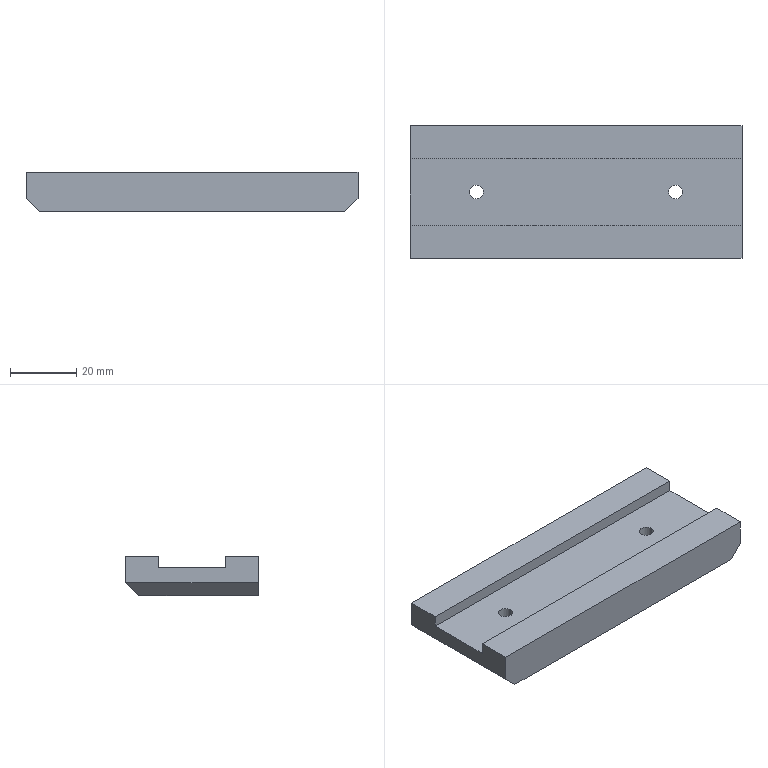Part | STEP file | X77-02103 | 1 solid | 17 faces | box 100 x 40 x 12 mm | volume 39367 mm3 | plane 13 | cylinder 4 | commonest cylinder face diameters 4.2 x4
STEP:
#1=CARTESIAN_POINT('',(-32.1,70.,0.));
#2=VERTEX_POINT('',#1);
#3=CARTESIAN_POINT('',(-27.9,70.,0.));
#4=VERTEX_POINT('',#3);
#5=CARTESIAN_POINT('',(-30.,70.,0.));
#6=DIRECTION('',(0.,0.,1.));
#7=DIRECTION('',(1.,0.,0.));
#8=AXIS2_PLACEMENT_3D('',#5,#6,#7);
#9=CIRCLE('',#8,2.1);
#10=EDGE_CURVE('',#2,#4,#9,.T.);
#11=ORIENTED_EDGE('',*,*,#10,.F.);
#12=CARTESIAN_POINT('',(-32.1,70.,8.5));
#13=VERTEX_POINT('',#12);
#14=CARTESIAN_POINT('',(-32.1,70.,8.5));
#15=DIRECTION('',(0.,0.,1.));
#16=VECTOR('',#15,1000.);
#17=LINE('',#14,#16);
#18=EDGE_CURVE('',#2,#13,#17,.T.);
#19=ORIENTED_EDGE('',*,*,#18,.T.);
#20=CARTESIAN_POINT('',(-27.9,70.,8.5));
#21=VERTEX_POINT('',#20);
#22=CARTESIAN_POINT('',(-30.,70.,8.5));
#23=DIRECTION('',(0.,0.,1.));
#24=DIRECTION('',(1.,0.,0.));
#25=AXIS2_PLACEMENT_3D('',#22,#23,#24);
#26=CIRCLE('',#25,2.1);
#27=EDGE_CURVE('',#13,#21,#26,.T.);
#28=ORIENTED_EDGE('',*,*,#27,.T.);
#29=CARTESIAN_POINT('',(-27.9,70.,8.5));
#30=DIRECTION('',(0.,0.,1.));
#31=VECTOR('',#30,1000.);
#32=LINE('',#29,#31);
#33=EDGE_CURVE('',#4,#21,#32,.T.);
#34=ORIENTED_EDGE('',*,*,#33,.F.);
#35=EDGE_LOOP('',(#11,#19,#28,#34));
#36=FACE_OUTER_BOUND('',#35,.T.);
#37=CARTESIAN_POINT('',(-30.,70.,8.5));
#38=DIRECTION('',(0.,0.,1.));
#39=DIRECTION('',(1.,0.,0.));
#40=AXIS2_PLACEMENT_3D('',#37,#38,#39);
#41=CYLINDRICAL_SURFACE('',#40,2.1);
#42=ADVANCED_FACE('',(#36),#41,.F.);
#43=CARTESIAN_POINT('',(27.9,70.,0.));
#44=VERTEX_POINT('',#43);
#45=CARTESIAN_POINT('',(32.1,70.,0.));
#46=VERTEX_POINT('',#45);
#47=CARTESIAN_POINT('',(30.,70.,0.));
#48=DIRECTION('',(0.,0.,1.));
#49=DIRECTION('',(1.,0.,0.));
#50=AXIS2_PLACEMENT_3D('',#47,#48,#49);
#51=CIRCLE('',#50,2.1);
#52=EDGE_CURVE('',#44,#46,#51,.T.);
#53=ORIENTED_EDGE('',*,*,#52,.F.);
#54=CARTESIAN_POINT('',(27.9,70.,8.5));
#55=VERTEX_POINT('',#54);
#56=CARTESIAN_POINT('',(27.9,70.,8.5));
#57=DIRECTION('',(0.,0.,1.));
#58=VECTOR('',#57,1000.);
#59=LINE('',#56,#58);
#60=EDGE_CURVE('',#44,#55,#59,.T.);
#61=ORIENTED_EDGE('',*,*,#60,.T.);
#62=CARTESIAN_POINT('',(32.1,70.,8.5));
#63=VERTEX_POINT('',#62);
#64=CARTESIAN_POINT('',(30.,70.,8.5));
#65=DIRECTION('',(0.,0.,1.));
#66=DIRECTION('',(1.,0.,0.));
#67=AXIS2_PLACEMENT_3D('',#64,#65,#66);
#68=CIRCLE('',#67,2.1);
#69=EDGE_CURVE('',#55,#63,#68,.T.);
#70=ORIENTED_EDGE('',*,*,#69,.T.);
#71=CARTESIAN_POINT('',(32.1,70.,8.5));
#72=DIRECTION('',(0.,0.,1.));
#73=VECTOR('',#72,1000.);
#74=LINE('',#71,#73);
#75=EDGE_CURVE('',#46,#63,#74,.T.);
#76=ORIENTED_EDGE('',*,*,#75,.F.);
#77=EDGE_LOOP('',(#53,#61,#70,#76));
#78=FACE_OUTER_BOUND('',#77,.T.);
#79=CARTESIAN_POINT('',(30.,70.,8.5));
#80=DIRECTION('',(0.,0.,1.));
#81=DIRECTION('',(1.,0.,0.));
#82=AXIS2_PLACEMENT_3D('',#79,#80,#81);
#83=CYLINDRICAL_SURFACE('',#82,2.1);
#84=ADVANCED_FACE('',(#78),#83,.F.);
#85=CARTESIAN_POINT('',(-50.,60.,12.));
#86=VERTEX_POINT('',#85);
#87=CARTESIAN_POINT('',(50.,60.,12.));
#88=VERTEX_POINT('',#87);
#89=CARTESIAN_POINT('',(-50.,60.,12.));
#90=DIRECTION('',(1.,0.,0.));
#91=VECTOR('',#90,1000.);
#92=LINE('',#89,#91);
#93=EDGE_CURVE('',#86,#88,#92,.T.);
#94=ORIENTED_EDGE('',*,*,#93,.F.);
#95=CARTESIAN_POINT('',(-50.,50.,12.));
#96=VERTEX_POINT('',#95);
#97=CARTESIAN_POINT('',(-50.,90.,12.));
#98=DIRECTION('',(0.,-1.,0.));
#99=VECTOR('',#98,1000.);
#100=LINE('',#97,#99);
#101=EDGE_CURVE('',#86,#96,#100,.T.);
#102=ORIENTED_EDGE('',*,*,#101,.T.);
#103=CARTESIAN_POINT('',(50.,50.,12.));
#104=VERTEX_POINT('',#103);
#105=CARTESIAN_POINT('',(-50.,50.,12.));
#106=DIRECTION('',(1.,0.,0.));
#107=VECTOR('',#106,1000.);
#108=LINE('',#105,#107);
#109=EDGE_CURVE('',#96,#104,#108,.T.);
#110=ORIENTED_EDGE('',*,*,#109,.T.);
#111=CARTESIAN_POINT('',(50.,90.,12.));
#112=DIRECTION('',(0.,1.,0.));
#113=VECTOR('',#112,1000.);
#114=LINE('',#111,#113);
#115=EDGE_CURVE('',#104,#88,#114,.T.);
#116=ORIENTED_EDGE('',*,*,#115,.T.);
#117=EDGE_LOOP('',(#94,#102,#110,#116));
#118=FACE_OUTER_BOUND('',#117,.T.);
#119=CARTESIAN_POINT('',(-50.,50.,12.));
#120=DIRECTION('',(0.,0.,1.));
#121=DIRECTION('',(1.,0.,0.));
#122=AXIS2_PLACEMENT_3D('',#119,#120,#121);
#123=PLANE('',#122);
#124=ADVANCED_FACE('',(#118),#123,.T.);
#125=ORIENTED_EDGE('',*,*,#101,.F.);
#126=CARTESIAN_POINT('',(-50.,60.,8.5));
#127=VERTEX_POINT('',#126);
#128=CARTESIAN_POINT('',(-50.,60.,8.5));
#129=DIRECTION('',(0.,0.,1.));
#130=VECTOR('',#129,1000.);
#131=LINE('',#128,#130);
#132=EDGE_CURVE('',#127,#86,#131,.T.);
#133=ORIENTED_EDGE('',*,*,#132,.F.);
#134=CARTESIAN_POINT('',(-50.,80.,8.5));
#135=VERTEX_POINT('',#134);
#136=CARTESIAN_POINT('',(-50.,80.,8.5));
#137=DIRECTION('',(0.,-1.,0.));
#138=VECTOR('',#137,1000.);
#139=LINE('',#136,#138);
#140=EDGE_CURVE('',#135,#127,#139,.T.);
#141=ORIENTED_EDGE('',*,*,#140,.F.);
#142=CARTESIAN_POINT('',(-50.,80.,12.));
#143=VERTEX_POINT('',#142);
#144=CARTESIAN_POINT('',(-50.,80.,8.5));
#145=DIRECTION('',(0.,0.,1.));
#146=VECTOR('',#145,1000.);
#147=LINE('',#144,#146);
#148=EDGE_CURVE('',#135,#143,#147,.T.);
#149=ORIENTED_EDGE('',*,*,#148,.T.);
#150=CARTESIAN_POINT('',(-50.,90.,12.));
#151=VERTEX_POINT('',#150);
#152=CARTESIAN_POINT('',(-50.,90.,12.));
#153=DIRECTION('',(0.,-1.,0.));
#154=VECTOR('',#153,1000.);
#155=LINE('',#152,#154);
#156=EDGE_CURVE('',#151,#143,#155,.T.);
#157=ORIENTED_EDGE('',*,*,#156,.F.);
#158=CARTESIAN_POINT('',(-50.,90.,4.));
#159=VERTEX_POINT('',#158);
#160=CARTESIAN_POINT('',(-50.,90.,12.));
#161=DIRECTION('',(0.,0.,-1.));
#162=VECTOR('',#161,1000.);
#163=LINE('',#160,#162);
#164=EDGE_CURVE('',#151,#159,#163,.T.);
#165=ORIENTED_EDGE('',*,*,#164,.T.);
#166=CARTESIAN_POINT('',(-50.,50.,4.));
#167=VERTEX_POINT('',#166);
#168=CARTESIAN_POINT('',(-50.,90.,4.));
#169=DIRECTION('',(0.,-1.,0.));
#170=VECTOR('',#169,1000.);
#171=LINE('',#168,#170);
#172=EDGE_CURVE('',#159,#167,#171,.T.);
#173=ORIENTED_EDGE('',*,*,#172,.T.);
#174=CARTESIAN_POINT('',(-50.,50.,12.));
#175=DIRECTION('',(0.,0.,-1.));
#176=VECTOR('',#175,1000.);
#177=LINE('',#174,#176);
#178=EDGE_CURVE('',#96,#167,#177,.T.);
#179=ORIENTED_EDGE('',*,*,#178,.F.);
#180=EDGE_LOOP('',(#125,#133,#141,#149,#157,#165,#173,#179));
#181=FACE_OUTER_BOUND('',#180,.T.);
#182=CARTESIAN_POINT('',(-50.,90.,12.));
#183=DIRECTION('',(1.,0.,0.));
#184=DIRECTION('',(0.,1.,0.));
#185=AXIS2_PLACEMENT_3D('',#182,#183,#184);
#186=PLANE('',#185);
#187=ADVANCED_FACE('',(#181),#186,.F.);
#188=ORIENTED_EDGE('',*,*,#178,.T.);
#189=CARTESIAN_POINT('',(-46.,50.,0.));
#190=VERTEX_POINT('',#189);
#191=CARTESIAN_POINT('',(-50.,50.,4.));
#192=DIRECTION('',(0.7071,0.,-0.7071));
#193=VECTOR('',#192,1000.);
#194=LINE('',#191,#193);
#195=EDGE_CURVE('',#167,#190,#194,.T.);
#196=ORIENTED_EDGE('',*,*,#195,.T.);
#197=CARTESIAN_POINT('',(46.,50.,0.));
#198=VERTEX_POINT('',#197);
#199=CARTESIAN_POINT('',(-50.,50.,0.));
#200=DIRECTION('',(1.,0.,0.));
#201=VECTOR('',#200,1000.);
#202=LINE('',#199,#201);
#203=EDGE_CURVE('',#190,#198,#202,.T.);
#204=ORIENTED_EDGE('',*,*,#203,.T.);
#205=CARTESIAN_POINT('',(50.,50.,4.));
#206=VERTEX_POINT('',#205);
#207=CARTESIAN_POINT('',(50.,50.,4.));
#208=DIRECTION('',(0.7071,0.,0.7071));
#209=VECTOR('',#208,1000.);
#210=LINE('',#207,#209);
#211=EDGE_CURVE('',#198,#206,#210,.T.);
#212=ORIENTED_EDGE('',*,*,#211,.T.);
#213=CARTESIAN_POINT('',(50.,50.,12.));
#214=DIRECTION('',(0.,0.,-1.));
#215=VECTOR('',#214,1000.);
#216=LINE('',#213,#215);
#217=EDGE_CURVE('',#104,#206,#216,.T.);
#218=ORIENTED_EDGE('',*,*,#217,.F.);
#219=ORIENTED_EDGE('',*,*,#109,.F.);
#220=EDGE_LOOP('',(#188,#196,#204,#212,#218,#219));
#221=FACE_OUTER_BOUND('',#220,.T.);
#222=CARTESIAN_POINT('',(-50.,50.,12.));
#223=DIRECTION('',(0.,1.,0.));
#224=DIRECTION('',(0.,0.,1.));
#225=AXIS2_PLACEMENT_3D('',#222,#223,#224);
#226=PLANE('',#225);
#227=ADVANCED_FACE('',(#221),#226,.F.);
#228=CARTESIAN_POINT('',(50.,60.,8.5));
#229=VERTEX_POINT('',#228);
#230=CARTESIAN_POINT('',(50.,80.,8.5));
#231=VERTEX_POINT('',#230);
#232=CARTESIAN_POINT('',(50.,80.,8.5));
#233=DIRECTION('',(0.,1.,0.));
#234=VECTOR('',#233,1000.);
#235=LINE('',#232,#234);
#236=EDGE_CURVE('',#229,#231,#235,.T.);
#237=ORIENTED_EDGE('',*,*,#236,.F.);
#238=CARTESIAN_POINT('',(50.,60.,8.5));
#239=DIRECTION('',(0.,0.,1.));
#240=VECTOR('',#239,1000.);
#241=LINE('',#238,#240);
#242=EDGE_CURVE('',#229,#88,#241,.T.);
#243=ORIENTED_EDGE('',*,*,#242,.T.);
#244=ORIENTED_EDGE('',*,*,#115,.F.);
#245=ORIENTED_EDGE('',*,*,#217,.T.);
#246=CARTESIAN_POINT('',(50.,90.,4.));
#247=VERTEX_POINT('',#246);
#248=CARTESIAN_POINT('',(50.,90.,4.));
#249=DIRECTION('',(0.,1.,0.));
#250=VECTOR('',#249,1000.);
#251=LINE('',#248,#250);
#252=EDGE_CURVE('',#206,#247,#251,.T.);
#253=ORIENTED_EDGE('',*,*,#252,.T.);
#254=CARTESIAN_POINT('',(50.,90.,12.));
#255=VERTEX_POINT('',#254);
#256=CARTESIAN_POINT('',(50.,90.,12.));
#257=DIRECTION('',(0.,0.,-1.));
#258=VECTOR('',#257,1000.);
#259=LINE('',#256,#258);
#260=EDGE_CURVE('',#255,#247,#259,.T.);
#261=ORIENTED_EDGE('',*,*,#260,.F.);
#262=CARTESIAN_POINT('',(50.,80.,12.));
#263=VERTEX_POINT('',#262);
#264=CARTESIAN_POINT('',(50.,90.,12.));
#265=DIRECTION('',(0.,1.,0.));
#266=VECTOR('',#265,1000.);
#267=LINE('',#264,#266);
#268=EDGE_CURVE('',#263,#255,#267,.T.);
#269=ORIENTED_EDGE('',*,*,#268,.F.);
#270=CARTESIAN_POINT('',(50.,80.,8.5));
#271=DIRECTION('',(0.,0.,1.));
#272=VECTOR('',#271,1000.);
#273=LINE('',#270,#272);
#274=EDGE_CURVE('',#231,#263,#273,.T.);
#275=ORIENTED_EDGE('',*,*,#274,.F.);
#276=EDGE_LOOP('',(#237,#243,#244,#245,#253,#261,#269,#275));
#277=FACE_OUTER_BOUND('',#276,.T.);
#278=CARTESIAN_POINT('',(50.,90.,12.));
#279=DIRECTION('',(-1.,0.,0.));
#280=DIRECTION('',(0.,0.,1.));
#281=AXIS2_PLACEMENT_3D('',#278,#279,#280);
#282=PLANE('',#281);
#283=ADVANCED_FACE('',(#277),#282,.F.);
#284=ORIENTED_EDGE('',*,*,#260,.T.);
#285=CARTESIAN_POINT('',(-50.,90.,4.));
#286=DIRECTION('',(-1.,0.,0.));
#287=VECTOR('',#286,1000.);
#288=LINE('',#285,#287);
#289=EDGE_CURVE('',#247,#159,#288,.T.);
#290=ORIENTED_EDGE('',*,*,#289,.T.);
#291=ORIENTED_EDGE('',*,*,#164,.F.);
#292=CARTESIAN_POINT('',(-50.,90.,12.));
#293=DIRECTION('',(-1.,0.,0.));
#294=VECTOR('',#293,1000.);
#295=LINE('',#292,#294);
#296=EDGE_CURVE('',#255,#151,#295,.T.);
#297=ORIENTED_EDGE('',*,*,#296,.F.);
#298=EDGE_LOOP('',(#284,#290,#291,#297));
#299=FACE_OUTER_BOUND('',#298,.T.);
#300=CARTESIAN_POINT('',(-50.,90.,12.));
#301=DIRECTION('',(0.,-1.,0.));
#302=DIRECTION('',(0.,0.,-1.));
#303=AXIS2_PLACEMENT_3D('',#300,#301,#302);
#304=PLANE('',#303);
#305=ADVANCED_FACE('',(#299),#304,.F.);
#306=CARTESIAN_POINT('',(-50.,80.,12.));
#307=DIRECTION('',(-1.,0.,0.));
#308=VECTOR('',#307,1000.);
#309=LINE('',#306,#308);
#310=EDGE_CURVE('',#263,#143,#309,.T.);
#311=ORIENTED_EDGE('',*,*,#310,.F.);
#312=ORIENTED_EDGE('',*,*,#268,.T.);
#313=ORIENTED_EDGE('',*,*,#296,.T.);
#314=ORIENTED_EDGE('',*,*,#156,.T.);
#315=EDGE_LOOP('',(#311,#312,#313,#314));
#316=FACE_OUTER_BOUND('',#315,.T.);
#317=CARTESIAN_POINT('',(-50.,50.,12.));
#318=DIRECTION('',(0.,0.,1.));
#319=DIRECTION('',(1.,0.,0.));
#320=AXIS2_PLACEMENT_3D('',#317,#318,#319);
#321=PLANE('',#320);
#322=ADVANCED_FACE('',(#316),#321,.T.);
#323=CARTESIAN_POINT('',(-30.,70.,0.));
#324=DIRECTION('',(0.,0.,1.));
#325=DIRECTION('',(1.,0.,0.));
#326=AXIS2_PLACEMENT_3D('',#323,#324,#325);
#327=CIRCLE('',#326,2.1);
#328=EDGE_CURVE('',#4,#2,#327,.T.);
#329=ORIENTED_EDGE('',*,*,#328,.T.);
#330=ORIENTED_EDGE('',*,*,#10,.T.);
#331=EDGE_LOOP('',(#329,#330));
#332=FACE_BOUND('',#331,.T.);
#333=CARTESIAN_POINT('',(30.,70.,0.));
#334=DIRECTION('',(0.,0.,1.));
#335=DIRECTION('',(1.,0.,0.));
#336=AXIS2_PLACEMENT_3D('',#333,#334,#335);
#337=CIRCLE('',#336,2.1);
#338=EDGE_CURVE('',#46,#44,#337,.T.);
#339=ORIENTED_EDGE('',*,*,#338,.T.);
#340=ORIENTED_EDGE('',*,*,#52,.T.);
#341=EDGE_LOOP('',(#339,#340));
#342=FACE_BOUND('',#341,.T.);
#343=ORIENTED_EDGE('',*,*,#203,.F.);
#344=CARTESIAN_POINT('',(-46.,86.,0.));
#345=VERTEX_POINT('',#344);
#346=CARTESIAN_POINT('',(-46.,50.,0.));
#347=DIRECTION('',(0.,1.,0.));
#348=VECTOR('',#347,1000.);
#349=LINE('',#346,#348);
#350=EDGE_CURVE('',#190,#345,#349,.T.);
#351=ORIENTED_EDGE('',*,*,#350,.T.);
#352=CARTESIAN_POINT('',(46.,86.,0.));
#353=VERTEX_POINT('',#352);
#354=CARTESIAN_POINT('',(-50.,86.,0.));
#355=DIRECTION('',(1.,0.,0.));
#356=VECTOR('',#355,1000.);
#357=LINE('',#354,#356);
#358=EDGE_CURVE('',#345,#353,#357,.T.);
#359=ORIENTED_EDGE('',*,*,#358,.T.);
#360=CARTESIAN_POINT('',(46.,50.,0.));
#361=DIRECTION('',(0.,-1.,0.));
#362=VECTOR('',#361,1000.);
#363=LINE('',#360,#362);
#364=EDGE_CURVE('',#353,#198,#363,.T.);
#365=ORIENTED_EDGE('',*,*,#364,.T.);
#366=EDGE_LOOP('',(#343,#351,#359,#365));
#367=FACE_OUTER_BOUND('',#366,.T.);
#368=CARTESIAN_POINT('',(-50.,50.,0.));
#369=DIRECTION('',(0.,0.,1.));
#370=DIRECTION('',(1.,0.,0.));
#371=AXIS2_PLACEMENT_3D('',#368,#369,#370);
#372=PLANE('',#371);
#373=ADVANCED_FACE('',(#332,#342,#367),#372,.F.);
#374=ORIENTED_EDGE('',*,*,#211,.F.);
#375=ORIENTED_EDGE('',*,*,#364,.F.);
#376=CARTESIAN_POINT('',(16.667,56.667,-29.333));
#377=DIRECTION('',(-0.5774,-0.5774,-0.5774));
#378=VECTOR('',#377,1000.);
#379=LINE('',#376,#378);
#380=EDGE_CURVE('',#247,#353,#379,.T.);
#381=ORIENTED_EDGE('',*,*,#380,.F.);
#382=ORIENTED_EDGE('',*,*,#252,.F.);
#383=EDGE_LOOP('',(#374,#375,#381,#382));
#384=FACE_OUTER_BOUND('',#383,.T.);
#385=CARTESIAN_POINT('',(50.,90.,4.));
#386=DIRECTION('',(-0.7071,0.,0.7071));
#387=DIRECTION('',(0.7071,0.,0.7071));
#388=AXIS2_PLACEMENT_3D('',#385,#386,#387);
#389=PLANE('',#388);
#390=ADVANCED_FACE('',(#384),#389,.F.);
#391=ORIENTED_EDGE('',*,*,#380,.T.);
#392=ORIENTED_EDGE('',*,*,#358,.F.);
#393=CARTESIAN_POINT('',(-50.,90.,4.));
#394=DIRECTION('',(0.5774,-0.5774,-0.5774));
#395=VECTOR('',#394,1000.);
#396=LINE('',#393,#395);
#397=EDGE_CURVE('',#159,#345,#396,.T.);
#398=ORIENTED_EDGE('',*,*,#397,.F.);
#399=ORIENTED_EDGE('',*,*,#289,.F.);
#400=EDGE_LOOP('',(#391,#392,#398,#399));
#401=FACE_OUTER_BOUND('',#400,.T.);
#402=CARTESIAN_POINT('',(-50.,90.,4.));
#403=DIRECTION('',(0.,-0.7071,0.7071));
#404=DIRECTION('',(0.,-0.7071,-0.7071));
#405=AXIS2_PLACEMENT_3D('',#402,#403,#404);
#406=PLANE('',#405);
#407=ADVANCED_FACE('',(#401),#406,.F.);
#408=ORIENTED_EDGE('',*,*,#397,.T.);
#409=ORIENTED_EDGE('',*,*,#350,.F.);
#410=ORIENTED_EDGE('',*,*,#195,.F.);
#411=ORIENTED_EDGE('',*,*,#172,.F.);
#412=EDGE_LOOP('',(#408,#409,#410,#411));
#413=FACE_OUTER_BOUND('',#412,.T.);
#414=CARTESIAN_POINT('',(-50.,90.,4.));
#415=DIRECTION('',(0.7071,0.,0.7071));
#416=DIRECTION('',(0.7071,0.,-0.7071));
#417=AXIS2_PLACEMENT_3D('',#414,#415,#416);
#418=PLANE('',#417);
#419=ADVANCED_FACE('',(#413),#418,.F.);
#420=ORIENTED_EDGE('',*,*,#93,.T.);
#421=ORIENTED_EDGE('',*,*,#242,.F.);
#422=CARTESIAN_POINT('',(-50.,60.,8.5));
#423=DIRECTION('',(1.,0.,0.));
#424=VECTOR('',#423,1000.);
#425=LINE('',#422,#424);
#426=EDGE_CURVE('',#127,#229,#425,.T.);
#427=ORIENTED_EDGE('',*,*,#426,.F.);
#428=ORIENTED_EDGE('',*,*,#132,.T.);
#429=EDGE_LOOP('',(#420,#421,#427,#428));
#430=FACE_OUTER_BOUND('',#429,.T.);
#431=CARTESIAN_POINT('',(-50.,60.,8.5));
#432=DIRECTION('',(0.,-1.,0.));
#433=DIRECTION('',(-1.,0.,0.));
#434=AXIS2_PLACEMENT_3D('',#431,#432,#433);
#435=PLANE('',#434);
#436=ADVANCED_FACE('',(#430),#435,.F.);
#437=ORIENTED_EDGE('',*,*,#310,.T.);
#438=ORIENTED_EDGE('',*,*,#148,.F.);
#439=CARTESIAN_POINT('',(-50.,80.,8.5));
#440=DIRECTION('',(-1.,0.,0.));
#441=VECTOR('',#440,1000.);
#442=LINE('',#439,#441);
#443=EDGE_CURVE('',#231,#135,#442,.T.);
#444=ORIENTED_EDGE('',*,*,#443,.F.);
#445=ORIENTED_EDGE('',*,*,#274,.T.);
#446=EDGE_LOOP('',(#437,#438,#444,#445));
#447=FACE_OUTER_BOUND('',#446,.T.);
#448=CARTESIAN_POINT('',(-50.,80.,8.5));
#449=DIRECTION('',(0.,1.,0.));
#450=DIRECTION('',(0.,0.,-1.));
#451=AXIS2_PLACEMENT_3D('',#448,#449,#450);
#452=PLANE('',#451);
#453=ADVANCED_FACE('',(#447),#452,.F.);
#454=CARTESIAN_POINT('',(-30.,70.,8.5));
#455=DIRECTION('',(0.,0.,1.));
#456=DIRECTION('',(1.,0.,0.));
#457=AXIS2_PLACEMENT_3D('',#454,#455,#456);
#458=CIRCLE('',#457,2.1);
#459=EDGE_CURVE('',#21,#13,#458,.T.);
#460=ORIENTED_EDGE('',*,*,#459,.F.);
#461=ORIENTED_EDGE('',*,*,#27,.F.);
#462=EDGE_LOOP('',(#460,#461));
#463=FACE_BOUND('',#462,.T.);
#464=CARTESIAN_POINT('',(30.,70.,8.5));
#465=DIRECTION('',(0.,0.,1.));
#466=DIRECTION('',(1.,0.,0.));
#467=AXIS2_PLACEMENT_3D('',#464,#465,#466);
#468=CIRCLE('',#467,2.1);
#469=EDGE_CURVE('',#63,#55,#468,.T.);
#470=ORIENTED_EDGE('',*,*,#469,.F.);
#471=ORIENTED_EDGE('',*,*,#69,.F.);
#472=EDGE_LOOP('',(#470,#471));
#473=FACE_BOUND('',#472,.T.);
#474=ORIENTED_EDGE('',*,*,#236,.T.);
#475=ORIENTED_EDGE('',*,*,#443,.T.);
#476=ORIENTED_EDGE('',*,*,#140,.T.);
#477=ORIENTED_EDGE('',*,*,#426,.T.);
#478=EDGE_LOOP('',(#474,#475,#476,#477));
#479=FACE_OUTER_BOUND('',#478,.T.);
#480=CARTESIAN_POINT('',(50.,60.,8.5));
#481=DIRECTION('',(0.,0.,1.));
#482=DIRECTION('',(1.,0.,0.));
#483=AXIS2_PLACEMENT_3D('',#480,#481,#482);
#484=PLANE('',#483);
#485=ADVANCED_FACE('',(#463,#473,#479),#484,.T.);
#486=ORIENTED_EDGE('',*,*,#60,.F.);
#487=ORIENTED_EDGE('',*,*,#338,.F.);
#488=ORIENTED_EDGE('',*,*,#75,.T.);
#489=ORIENTED_EDGE('',*,*,#469,.T.);
#490=EDGE_LOOP('',(#486,#487,#488,#489));
#491=FACE_OUTER_BOUND('',#490,.T.);
#492=CARTESIAN_POINT('',(30.,70.,8.5));
#493=DIRECTION('',(0.,0.,1.));
#494=DIRECTION('',(1.,0.,0.));
#495=AXIS2_PLACEMENT_3D('',#492,#493,#494);
#496=CYLINDRICAL_SURFACE('',#495,2.1);
#497=ADVANCED_FACE('',(#491),#496,.F.);
#498=ORIENTED_EDGE('',*,*,#18,.F.);
#499=ORIENTED_EDGE('',*,*,#328,.F.);
#500=ORIENTED_EDGE('',*,*,#33,.T.);
#501=ORIENTED_EDGE('',*,*,#459,.T.);
#502=EDGE_LOOP('',(#498,#499,#500,#501));
#503=FACE_OUTER_BOUND('',#502,.T.);
#504=CARTESIAN_POINT('',(-30.,70.,8.5));
#505=DIRECTION('',(0.,0.,1.));
#506=DIRECTION('',(1.,0.,0.));
#507=AXIS2_PLACEMENT_3D('',#504,#505,#506);
#508=CYLINDRICAL_SURFACE('',#507,2.1);
#509=ADVANCED_FACE('',(#503),#508,.F.);
#510=CLOSED_SHELL('',(#42,#84,#124,#187,#227,#283,#305,#322,#373,#390,#407,#419,#436,#453,#485,#497,#509));
#511=MANIFOLD_SOLID_BREP('',#510);
#512=CARTESIAN_POINT('',(0.,0.,0.));
#513=DIRECTION('',(0.,0.,1.));
#514=DIRECTION('',(1.,0.,0.));
#515=AXIS2_PLACEMENT_3D('',#512,#513,#514);
#516=(LENGTH_UNIT()NAMED_UNIT(*)SI_UNIT(.MILLI.,.METRE.));
#517=UNCERTAINTY_MEASURE_WITH_UNIT(LENGTH_MEASURE(0.00001),#516,'','');
#518=(NAMED_UNIT(*)PLANE_ANGLE_UNIT()SI_UNIT($,.RADIAN.));
#519=(NAMED_UNIT(*)SI_UNIT($,.STERADIAN.)SOLID_ANGLE_UNIT());
#520=(GEOMETRIC_REPRESENTATION_CONTEXT(3)GLOBAL_UNCERTAINTY_ASSIGNED_CONTEXT((#517))GLOBAL_UNIT_ASSIGNED_CONTEXT((#516,#518,#519))REPRESENTATION_CONTEXT('',''));
#521=ADVANCED_BREP_SHAPE_REPRESENTATION('',(#511,#515),#520);